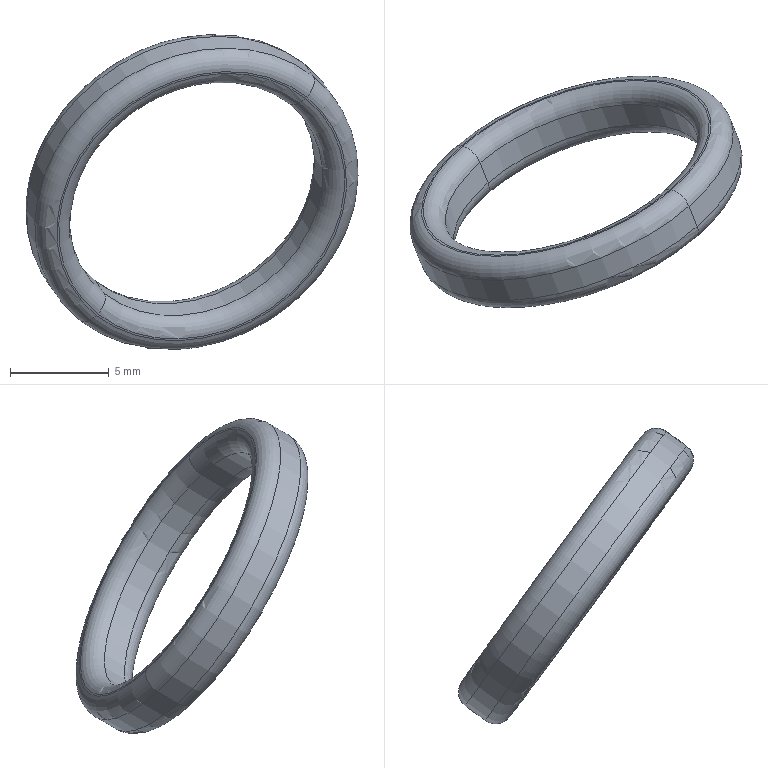Part | SolidWorks | features BaseBody 1 | 1 solid | 14 faces | box 16.862 x 11.769 x 16.004 mm | volume 237.71 mm3 | torus 8 | cylinder 4 | plane 2 | commonest cylinder face diameters 13.6 x2 17.3 x2
STEP:
#1=CARTESIAN_POINT('',(1927.105,-162.275,937.682));
#2=VERTEX_POINT('',#1);
#3=CARTESIAN_POINT('',(1926.789,-162.862,936.64));
#4=VERTEX_POINT('',#3);
#5=CARTESIAN_POINT('',(1926.504,-162.149,937.059));
#6=DIRECTION('',(0.6502,0.5603,-0.5131));
#7=DIRECTION('',(-0.3253,0.8156,0.4784));
#8=AXIS2_PLACEMENT_3D('',#5,#6,#7);
#9=CIRCLE('',#8,0.875);
#10=EDGE_CURVE('',#2,#4,#9,.T.);
#11=ORIENTED_EDGE('',*,*,#10,.T.);
#12=CARTESIAN_POINT('',(1937.327,-165.075,947.579));
#13=VERTEX_POINT('',#12);
#14=CARTESIAN_POINT('',(1932.058,-163.969,942.109));
#15=DIRECTION('',(-0.3253,0.8156,0.4784));
#16=DIRECTION('',(-0.8998,-0.4226,0.1086));
#17=AXIS2_PLACEMENT_3D('',#14,#15,#16);
#18=CIRCLE('',#17,7.675);
#19=EDGE_CURVE('',#13,#4,#18,.T.);
#20=ORIENTED_EDGE('',*,*,#19,.F.);
#21=CARTESIAN_POINT('',(1936.442,-164.235,947.374));
#22=VERTEX_POINT('',#21);
#23=CARTESIAN_POINT('',(1937.043,-164.362,947.998));
#24=DIRECTION('',(0.6502,0.5603,-0.5131));
#25=DIRECTION('',(-0.3253,0.8156,0.4784));
#26=AXIS2_PLACEMENT_3D('',#23,#24,#25);
#27=CIRCLE('',#26,0.875);
#28=EDGE_CURVE('',#13,#22,#27,.T.);
#29=ORIENTED_EDGE('',*,*,#28,.T.);
#30=CARTESIAN_POINT('',(1931.773,-163.255,942.528));
#31=DIRECTION('',(-0.3253,0.8156,0.4784));
#32=DIRECTION('',(-0.8998,-0.4226,0.1086));
#33=AXIS2_PLACEMENT_3D('',#30,#31,#32);
#34=CIRCLE('',#33,6.8);
#35=EDGE_CURVE('',#22,#2,#34,.T.);
#36=ORIENTED_EDGE('',*,*,#35,.T.);
#37=EDGE_LOOP('',(#11,#20,#29,#36));
#38=FACE_OUTER_BOUND('',#37,.T.);
#39=CARTESIAN_POINT('',(1931.773,-163.255,942.528));
#40=DIRECTION('',(-0.3253,0.8156,0.4784));
#41=DIRECTION('',(-0.6866,0.1442,-0.7126));
#42=AXIS2_PLACEMENT_3D('',#39,#40,#41);
#43=TOROIDAL_SURFACE('',#42,7.675,0.875);
#44=ADVANCED_FACE('',(#38),#43,.T.);
#45=ORIENTED_EDGE('',*,*,#28,.F.);
#46=CARTESIAN_POINT('',(1932.058,-163.969,942.109));
#47=DIRECTION('',(-0.3253,0.8156,0.4784));
#48=DIRECTION('',(-0.8998,-0.4226,0.1086));
#49=AXIS2_PLACEMENT_3D('',#46,#47,#48);
#50=CIRCLE('',#49,7.675);
#51=EDGE_CURVE('',#4,#13,#50,.T.);
#52=ORIENTED_EDGE('',*,*,#51,.F.);
#53=ORIENTED_EDGE('',*,*,#10,.F.);
#54=CARTESIAN_POINT('',(1931.773,-163.255,942.528));
#55=DIRECTION('',(-0.3253,0.8156,0.4784));
#56=DIRECTION('',(-0.8998,-0.4226,0.1086));
#57=AXIS2_PLACEMENT_3D('',#54,#55,#56);
#58=CIRCLE('',#57,6.8);
#59=EDGE_CURVE('',#2,#22,#58,.T.);
#60=ORIENTED_EDGE('',*,*,#59,.T.);
#61=EDGE_LOOP('',(#45,#52,#53,#60));
#62=FACE_OUTER_BOUND('',#61,.T.);
#63=CARTESIAN_POINT('',(1931.773,-163.255,942.528));
#64=DIRECTION('',(-0.3253,0.8156,0.4784));
#65=DIRECTION('',(-0.6866,0.1442,-0.7126));
#66=AXIS2_PLACEMENT_3D('',#63,#64,#65);
#67=TOROIDAL_SURFACE('',#66,7.675,0.875);
#68=ADVANCED_FACE('',(#62),#67,.T.);
#69=CARTESIAN_POINT('',(1926.697,-161.253,938.281));
#70=VERTEX_POINT('',#69);
#71=CARTESIAN_POINT('',(1926.901,-161.764,937.982));
#72=DIRECTION('',(0.3253,-0.8156,-0.4784));
#73=VECTOR('',#72,1000.);
#74=LINE('',#71,#73);
#75=EDGE_CURVE('',#70,#2,#74,.T.);
#76=ORIENTED_EDGE('',*,*,#75,.T.);
#77=ORIENTED_EDGE('',*,*,#35,.F.);
#78=CARTESIAN_POINT('',(1936.034,-163.214,947.973));
#79=VERTEX_POINT('',#78);
#80=CARTESIAN_POINT('',(1936.238,-163.725,947.674));
#81=DIRECTION('',(-0.3253,0.8156,0.4784));
#82=VECTOR('',#81,1000.);
#83=LINE('',#80,#82);
#84=EDGE_CURVE('',#22,#79,#83,.T.);
#85=ORIENTED_EDGE('',*,*,#84,.T.);
#86=CARTESIAN_POINT('',(1931.366,-162.234,943.127));
#87=DIRECTION('',(-0.3253,0.8156,0.4784));
#88=DIRECTION('',(-0.8998,-0.4226,0.1086));
#89=AXIS2_PLACEMENT_3D('',#86,#87,#88);
#90=CIRCLE('',#89,6.8);
#91=EDGE_CURVE('',#79,#70,#90,.T.);
#92=ORIENTED_EDGE('',*,*,#91,.T.);
#93=EDGE_LOOP('',(#76,#77,#85,#92));
#94=FACE_OUTER_BOUND('',#93,.T.);
#95=CARTESIAN_POINT('',(1931.57,-162.744,942.828));
#96=DIRECTION('',(-0.3253,0.8156,0.4784));
#97=DIRECTION('',(-0.6866,0.1442,-0.7126));
#98=AXIS2_PLACEMENT_3D('',#95,#96,#97);
#99=CYLINDRICAL_SURFACE('',#98,6.8);
#100=ADVANCED_FACE('',(#94),#99,.F.);
#101=ORIENTED_EDGE('',*,*,#84,.F.);
#102=ORIENTED_EDGE('',*,*,#59,.F.);
#103=ORIENTED_EDGE('',*,*,#75,.F.);
#104=CARTESIAN_POINT('',(1931.366,-162.234,943.127));
#105=DIRECTION('',(-0.3253,0.8156,0.4784));
#106=DIRECTION('',(-0.8998,-0.4226,0.1086));
#107=AXIS2_PLACEMENT_3D('',#104,#105,#106);
#108=CIRCLE('',#107,6.8);
#109=EDGE_CURVE('',#70,#79,#108,.T.);
#110=ORIENTED_EDGE('',*,*,#109,.T.);
#111=EDGE_LOOP('',(#101,#102,#103,#110));
#112=FACE_OUTER_BOUND('',#111,.T.);
#113=CARTESIAN_POINT('',(1931.57,-162.744,942.828));
#114=DIRECTION('',(-0.3253,0.8156,0.4784));
#115=DIRECTION('',(-0.6866,0.1442,-0.7126));
#116=AXIS2_PLACEMENT_3D('',#113,#114,#115);
#117=CYLINDRICAL_SURFACE('',#116,6.8);
#118=ADVANCED_FACE('',(#112),#117,.F.);
#119=CARTESIAN_POINT('',(1925.812,-160.413,938.076));
#120=VERTEX_POINT('',#119);
#121=CARTESIAN_POINT('',(1926.097,-161.127,937.658));
#122=DIRECTION('',(0.6502,0.5603,-0.5131));
#123=DIRECTION('',(-0.3253,0.8156,0.4784));
#124=AXIS2_PLACEMENT_3D('',#121,#122,#123);
#125=CIRCLE('',#124,0.875);
#126=EDGE_CURVE('',#120,#70,#125,.T.);
#127=ORIENTED_EDGE('',*,*,#126,.T.);
#128=ORIENTED_EDGE('',*,*,#91,.F.);
#129=CARTESIAN_POINT('',(1936.351,-162.626,949.015));
#130=VERTEX_POINT('',#129);
#131=CARTESIAN_POINT('',(1936.635,-163.34,948.597));
#132=DIRECTION('',(0.6502,0.5603,-0.5131));
#133=DIRECTION('',(-0.3253,0.8156,0.4784));
#134=AXIS2_PLACEMENT_3D('',#131,#132,#133);
#135=CIRCLE('',#134,0.875);
#136=EDGE_CURVE('',#79,#130,#135,.T.);
#137=ORIENTED_EDGE('',*,*,#136,.T.);
#138=CARTESIAN_POINT('',(1931.081,-161.52,943.546));
#139=DIRECTION('',(-0.3253,0.8156,0.4784));
#140=DIRECTION('',(-0.8998,-0.4226,0.1086));
#141=AXIS2_PLACEMENT_3D('',#138,#139,#140);
#142=CIRCLE('',#141,7.675);
#143=EDGE_CURVE('',#130,#120,#142,.T.);
#144=ORIENTED_EDGE('',*,*,#143,.T.);
#145=EDGE_LOOP('',(#127,#128,#137,#144));
#146=FACE_OUTER_BOUND('',#145,.T.);
#147=CARTESIAN_POINT('',(1931.366,-162.234,943.127));
#148=DIRECTION('',(-0.3253,0.8156,0.4784));
#149=DIRECTION('',(-0.6866,0.1442,-0.7126));
#150=AXIS2_PLACEMENT_3D('',#147,#148,#149);
#151=TOROIDAL_SURFACE('',#150,7.675,0.875);
#152=ADVANCED_FACE('',(#146),#151,.T.);
#153=ORIENTED_EDGE('',*,*,#136,.F.);
#154=ORIENTED_EDGE('',*,*,#109,.F.);
#155=ORIENTED_EDGE('',*,*,#126,.F.);
#156=CARTESIAN_POINT('',(1931.081,-161.52,943.546));
#157=DIRECTION('',(-0.3253,0.8156,0.4784));
#158=DIRECTION('',(-0.8998,-0.4226,0.1086));
#159=AXIS2_PLACEMENT_3D('',#156,#157,#158);
#160=CIRCLE('',#159,7.675);
#161=EDGE_CURVE('',#120,#130,#160,.T.);
#162=ORIENTED_EDGE('',*,*,#161,.T.);
#163=EDGE_LOOP('',(#153,#154,#155,#162));
#164=FACE_OUTER_BOUND('',#163,.T.);
#165=CARTESIAN_POINT('',(1931.366,-162.234,943.127));
#166=DIRECTION('',(-0.3253,0.8156,0.4784));
#167=DIRECTION('',(-0.6866,0.1442,-0.7126));
#168=AXIS2_PLACEMENT_3D('',#165,#166,#167);
#169=TOROIDAL_SURFACE('',#168,7.675,0.875);
#170=ADVANCED_FACE('',(#164),#169,.T.);
#171=CARTESIAN_POINT('',(1925.427,-160.986,936.963));
#172=VERTEX_POINT('',#171);
#173=CARTESIAN_POINT('',(1925.743,-160.399,938.005));
#174=VERTEX_POINT('',#173);
#175=CARTESIAN_POINT('',(1926.028,-161.113,937.587));
#176=DIRECTION('',(0.6502,0.5603,-0.5131));
#177=DIRECTION('',(-0.3253,0.8156,0.4784));
#178=AXIS2_PLACEMENT_3D('',#175,#176,#177);
#179=CIRCLE('',#178,0.875);
#180=EDGE_CURVE('',#172,#174,#179,.T.);
#181=ORIENTED_EDGE('',*,*,#180,.T.);
#182=CARTESIAN_POINT('',(1936.419,-162.641,949.087));
#183=VERTEX_POINT('',#182);
#184=CARTESIAN_POINT('',(1931.081,-161.52,943.546));
#185=DIRECTION('',(-0.3253,0.8156,0.4784));
#186=DIRECTION('',(-0.8998,-0.4226,0.1086));
#187=AXIS2_PLACEMENT_3D('',#184,#185,#186);
#188=CIRCLE('',#187,7.775);
#189=EDGE_CURVE('',#183,#174,#188,.T.);
#190=ORIENTED_EDGE('',*,*,#189,.F.);
#191=CARTESIAN_POINT('',(1937.305,-163.481,949.292));
#192=VERTEX_POINT('',#191);
#193=CARTESIAN_POINT('',(1936.704,-163.354,948.668));
#194=DIRECTION('',(0.6502,0.5603,-0.5131));
#195=DIRECTION('',(-0.3253,0.8156,0.4784));
#196=AXIS2_PLACEMENT_3D('',#193,#194,#195);
#197=CIRCLE('',#196,0.875);
#198=EDGE_CURVE('',#183,#192,#197,.T.);
#199=ORIENTED_EDGE('',*,*,#198,.T.);
#200=CARTESIAN_POINT('',(1931.366,-162.234,943.127));
#201=DIRECTION('',(-0.3253,0.8156,0.4784));
#202=DIRECTION('',(-0.8998,-0.4226,0.1086));
#203=AXIS2_PLACEMENT_3D('',#200,#201,#202);
#204=CIRCLE('',#203,8.65);
#205=EDGE_CURVE('',#192,#172,#204,.T.);
#206=ORIENTED_EDGE('',*,*,#205,.T.);
#207=EDGE_LOOP('',(#181,#190,#199,#206));
#208=FACE_OUTER_BOUND('',#207,.T.);
#209=CARTESIAN_POINT('',(1931.366,-162.234,943.127));
#210=DIRECTION('',(-0.3253,0.8156,0.4784));
#211=DIRECTION('',(-0.6866,0.1442,-0.7126));
#212=AXIS2_PLACEMENT_3D('',#209,#210,#211);
#213=TOROIDAL_SURFACE('',#212,7.775,0.875);
#214=ADVANCED_FACE('',(#208),#213,.T.);
#215=ORIENTED_EDGE('',*,*,#198,.F.);
#216=CARTESIAN_POINT('',(1931.081,-161.52,943.546));
#217=DIRECTION('',(-0.3253,0.8156,0.4784));
#218=DIRECTION('',(-0.8998,-0.4226,0.1086));
#219=AXIS2_PLACEMENT_3D('',#216,#217,#218);
#220=CIRCLE('',#219,7.775);
#221=EDGE_CURVE('',#174,#183,#220,.T.);
#222=ORIENTED_EDGE('',*,*,#221,.F.);
#223=ORIENTED_EDGE('',*,*,#180,.F.);
#224=CARTESIAN_POINT('',(1931.366,-162.234,943.127));
#225=DIRECTION('',(-0.3253,0.8156,0.4784));
#226=DIRECTION('',(-0.8998,-0.4226,0.1086));
#227=AXIS2_PLACEMENT_3D('',#224,#225,#226);
#228=CIRCLE('',#227,8.65);
#229=EDGE_CURVE('',#172,#192,#228,.T.);
#230=ORIENTED_EDGE('',*,*,#229,.T.);
#231=EDGE_LOOP('',(#215,#222,#223,#230));
#232=FACE_OUTER_BOUND('',#231,.T.);
#233=CARTESIAN_POINT('',(1931.366,-162.234,943.127));
#234=DIRECTION('',(-0.3253,0.8156,0.4784));
#235=DIRECTION('',(-0.6866,0.1442,-0.7126));
#236=AXIS2_PLACEMENT_3D('',#233,#234,#235);
#237=TOROIDAL_SURFACE('',#236,7.775,0.875);
#238=ADVANCED_FACE('',(#232),#237,.T.);
#239=CARTESIAN_POINT('',(1925.835,-162.008,936.364));
#240=VERTEX_POINT('',#239);
#241=CARTESIAN_POINT('',(1925.631,-161.497,936.663));
#242=DIRECTION('',(-0.3253,0.8156,0.4784));
#243=VECTOR('',#242,1000.);
#244=LINE('',#241,#243);
#245=EDGE_CURVE('',#240,#172,#244,.T.);
#246=ORIENTED_EDGE('',*,*,#245,.T.);
#247=ORIENTED_EDGE('',*,*,#205,.F.);
#248=CARTESIAN_POINT('',(1937.712,-164.502,948.692));
#249=VERTEX_POINT('',#248);
#250=CARTESIAN_POINT('',(1937.508,-163.991,948.992));
#251=DIRECTION('',(0.3253,-0.8156,-0.4784));
#252=VECTOR('',#251,1000.);
#253=LINE('',#250,#252);
#254=EDGE_CURVE('',#192,#249,#253,.T.);
#255=ORIENTED_EDGE('',*,*,#254,.T.);
#256=CARTESIAN_POINT('',(1931.773,-163.255,942.528));
#257=DIRECTION('',(-0.3253,0.8156,0.4784));
#258=DIRECTION('',(-0.8998,-0.4226,0.1086));
#259=AXIS2_PLACEMENT_3D('',#256,#257,#258);
#260=CIRCLE('',#259,8.65);
#261=EDGE_CURVE('',#249,#240,#260,.T.);
#262=ORIENTED_EDGE('',*,*,#261,.T.);
#263=EDGE_LOOP('',(#246,#247,#255,#262));
#264=FACE_OUTER_BOUND('',#263,.T.);
#265=CARTESIAN_POINT('',(1931.57,-162.744,942.828));
#266=DIRECTION('',(-0.3253,0.8156,0.4784));
#267=DIRECTION('',(-0.6866,0.1442,-0.7126));
#268=AXIS2_PLACEMENT_3D('',#265,#266,#267);
#269=CYLINDRICAL_SURFACE('',#268,8.65);
#270=ADVANCED_FACE('',(#264),#269,.T.);
#271=ORIENTED_EDGE('',*,*,#254,.F.);
#272=ORIENTED_EDGE('',*,*,#229,.F.);
#273=ORIENTED_EDGE('',*,*,#245,.F.);
#274=CARTESIAN_POINT('',(1931.773,-163.255,942.528));
#275=DIRECTION('',(-0.3253,0.8156,0.4784));
#276=DIRECTION('',(-0.8998,-0.4226,0.1086));
#277=AXIS2_PLACEMENT_3D('',#274,#275,#276);
#278=CIRCLE('',#277,8.65);
#279=EDGE_CURVE('',#240,#249,#278,.T.);
#280=ORIENTED_EDGE('',*,*,#279,.T.);
#281=EDGE_LOOP('',(#271,#272,#273,#280));
#282=FACE_OUTER_BOUND('',#281,.T.);
#283=CARTESIAN_POINT('',(1931.57,-162.744,942.828));
#284=DIRECTION('',(-0.3253,0.8156,0.4784));
#285=DIRECTION('',(-0.6866,0.1442,-0.7126));
#286=AXIS2_PLACEMENT_3D('',#283,#284,#285);
#287=CYLINDRICAL_SURFACE('',#286,8.65);
#288=ADVANCED_FACE('',(#282),#287,.T.);
#289=CARTESIAN_POINT('',(1926.72,-162.848,936.569));
#290=VERTEX_POINT('',#289);
#291=CARTESIAN_POINT('',(1926.435,-162.134,936.987));
#292=DIRECTION('',(0.6502,0.5603,-0.5131));
#293=DIRECTION('',(-0.3253,0.8156,0.4784));
#294=AXIS2_PLACEMENT_3D('',#291,#292,#293);
#295=CIRCLE('',#294,0.875);
#296=EDGE_CURVE('',#290,#240,#295,.T.);
#297=ORIENTED_EDGE('',*,*,#296,.T.);
#298=ORIENTED_EDGE('',*,*,#261,.F.);
#299=CARTESIAN_POINT('',(1937.396,-165.09,947.65));
#300=VERTEX_POINT('',#299);
#301=CARTESIAN_POINT('',(1937.111,-164.376,948.069));
#302=DIRECTION('',(0.6502,0.5603,-0.5131));
#303=DIRECTION('',(-0.3253,0.8156,0.4784));
#304=AXIS2_PLACEMENT_3D('',#301,#302,#303);
#305=CIRCLE('',#304,0.875);
#306=EDGE_CURVE('',#249,#300,#305,.T.);
#307=ORIENTED_EDGE('',*,*,#306,.T.);
#308=CARTESIAN_POINT('',(1932.058,-163.969,942.109));
#309=DIRECTION('',(-0.3253,0.8156,0.4784));
#310=DIRECTION('',(-0.8998,-0.4226,0.1086));
#311=AXIS2_PLACEMENT_3D('',#308,#309,#310);
#312=CIRCLE('',#311,7.775);
#313=EDGE_CURVE('',#300,#290,#312,.T.);
#314=ORIENTED_EDGE('',*,*,#313,.T.);
#315=EDGE_LOOP('',(#297,#298,#307,#314));
#316=FACE_OUTER_BOUND('',#315,.T.);
#317=CARTESIAN_POINT('',(1931.773,-163.255,942.528));
#318=DIRECTION('',(-0.3253,0.8156,0.4784));
#319=DIRECTION('',(-0.6866,0.1442,-0.7126));
#320=AXIS2_PLACEMENT_3D('',#317,#318,#319);
#321=TOROIDAL_SURFACE('',#320,7.775,0.875);
#322=ADVANCED_FACE('',(#316),#321,.T.);
#323=ORIENTED_EDGE('',*,*,#306,.F.);
#324=ORIENTED_EDGE('',*,*,#279,.F.);
#325=ORIENTED_EDGE('',*,*,#296,.F.);
#326=CARTESIAN_POINT('',(1932.058,-163.969,942.109));
#327=DIRECTION('',(-0.3253,0.8156,0.4784));
#328=DIRECTION('',(-0.8998,-0.4226,0.1086));
#329=AXIS2_PLACEMENT_3D('',#326,#327,#328);
#330=CIRCLE('',#329,7.775);
#331=EDGE_CURVE('',#290,#300,#330,.T.);
#332=ORIENTED_EDGE('',*,*,#331,.T.);
#333=EDGE_LOOP('',(#323,#324,#325,#332));
#334=FACE_OUTER_BOUND('',#333,.T.);
#335=CARTESIAN_POINT('',(1931.773,-163.255,942.528));
#336=DIRECTION('',(-0.3253,0.8156,0.4784));
#337=DIRECTION('',(-0.6866,0.1442,-0.7126));
#338=AXIS2_PLACEMENT_3D('',#335,#336,#337);
#339=TOROIDAL_SURFACE('',#338,7.775,0.875);
#340=ADVANCED_FACE('',(#334),#339,.T.);
#341=ORIENTED_EDGE('',*,*,#313,.F.);
#342=ORIENTED_EDGE('',*,*,#331,.F.);
#343=EDGE_LOOP('',(#341,#342));
#344=FACE_OUTER_BOUND('',#343,.T.);
#345=ORIENTED_EDGE('',*,*,#51,.T.);
#346=ORIENTED_EDGE('',*,*,#19,.T.);
#347=EDGE_LOOP('',(#345,#346));
#348=FACE_BOUND('',#347,.T.);
#349=CARTESIAN_POINT('',(1934.29,-167.002,948.797));
#350=DIRECTION('',(-0.3253,0.8156,0.4784));
#351=DIRECTION('',(-0.2908,0.3952,-0.8714));
#352=AXIS2_PLACEMENT_3D('',#349,#350,#351);
#353=PLANE('',#352);
#354=ADVANCED_FACE('',(#344,#348),#353,.F.);
#355=ORIENTED_EDGE('',*,*,#221,.T.);
#356=ORIENTED_EDGE('',*,*,#189,.T.);
#357=EDGE_LOOP('',(#355,#356));
#358=FACE_OUTER_BOUND('',#357,.T.);
#359=ORIENTED_EDGE('',*,*,#143,.F.);
#360=ORIENTED_EDGE('',*,*,#161,.F.);
#361=EDGE_LOOP('',(#359,#360));
#362=FACE_BOUND('',#361,.T.);
#363=CARTESIAN_POINT('',(1933.342,-164.592,950.321));
#364=DIRECTION('',(-0.3253,0.8156,0.4784));
#365=DIRECTION('',(-0.2908,0.3952,-0.8714));
#366=AXIS2_PLACEMENT_3D('',#363,#364,#365);
#367=PLANE('',#366);
#368=ADVANCED_FACE('',(#358,#362),#367,.T.);
#369=CLOSED_SHELL('',(#44,#68,#100,#118,#152,#170,#214,#238,#270,#288,#322,#340,#354,#368));
#370=MANIFOLD_SOLID_BREP('',#369);
#371=CARTESIAN_POINT('',(0.,0.,0.));
#372=DIRECTION('',(0.,0.,1.));
#373=DIRECTION('',(1.,0.,0.));
#374=AXIS2_PLACEMENT_3D('',#371,#372,#373);
#375=(LENGTH_UNIT()NAMED_UNIT(*)SI_UNIT(.MILLI.,.METRE.));
#376=UNCERTAINTY_MEASURE_WITH_UNIT(LENGTH_MEASURE(0.00001),#375,'','');
#377=(NAMED_UNIT(*)PLANE_ANGLE_UNIT()SI_UNIT($,.RADIAN.));
#378=(NAMED_UNIT(*)SI_UNIT($,.STERADIAN.)SOLID_ANGLE_UNIT());
#379=(GEOMETRIC_REPRESENTATION_CONTEXT(3)GLOBAL_UNCERTAINTY_ASSIGNED_CONTEXT((#376))GLOBAL_UNIT_ASSIGNED_CONTEXT((#375,#377,#378))REPRESENTATION_CONTEXT('',''));
#380=ADVANCED_BREP_SHAPE_REPRESENTATION('',(#370,#374),#379);